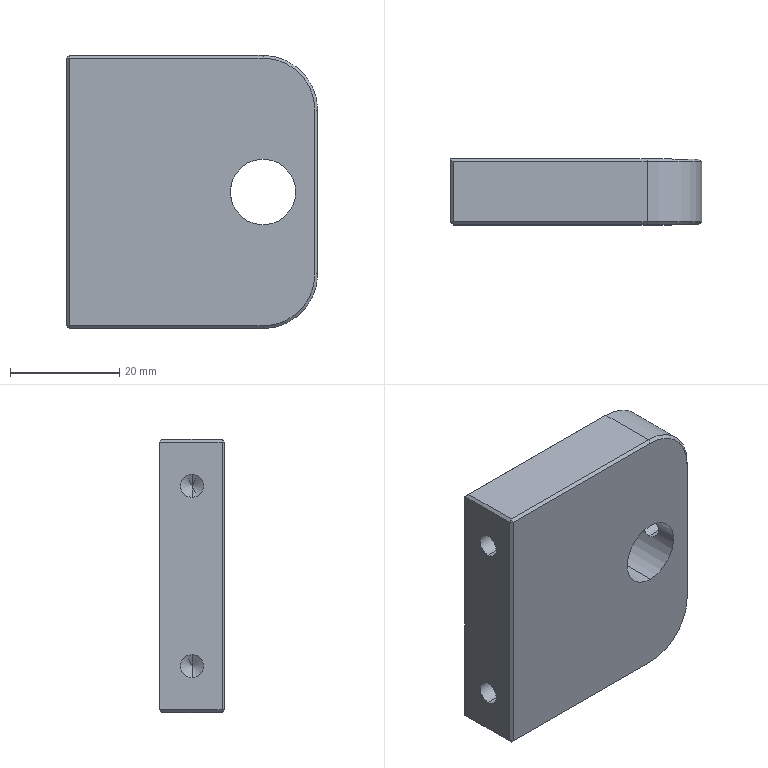Part | STEP file | ND25021-01-JDKM-53-TL | 1 solid | 37 faces | box 46 x 12 x 50 mm | volume 25274 mm3 | plane 17 | cylinder 10 | cone 10 | commonest cylinder face diameters 4.2 x6 12 x2 20 x2